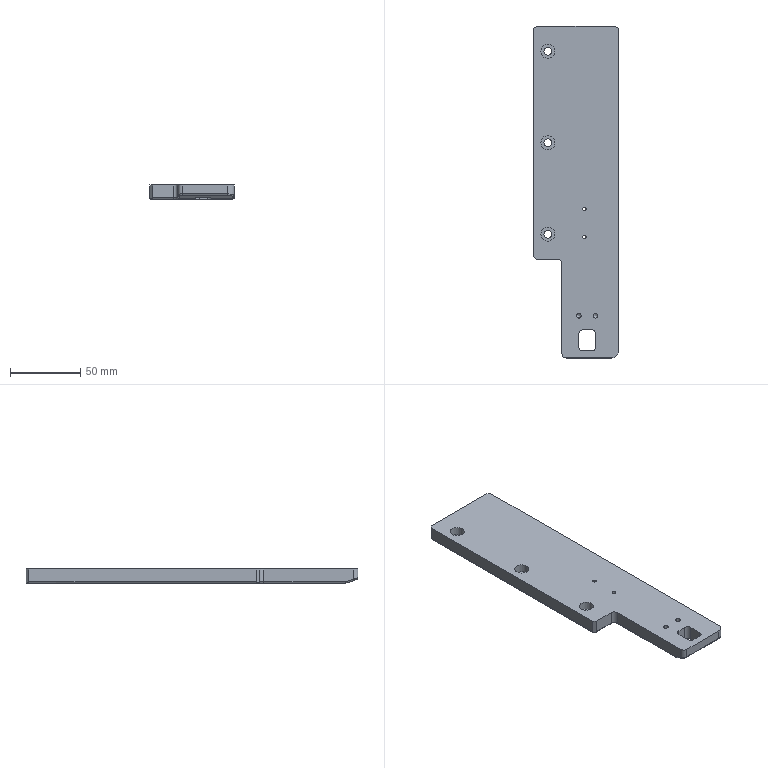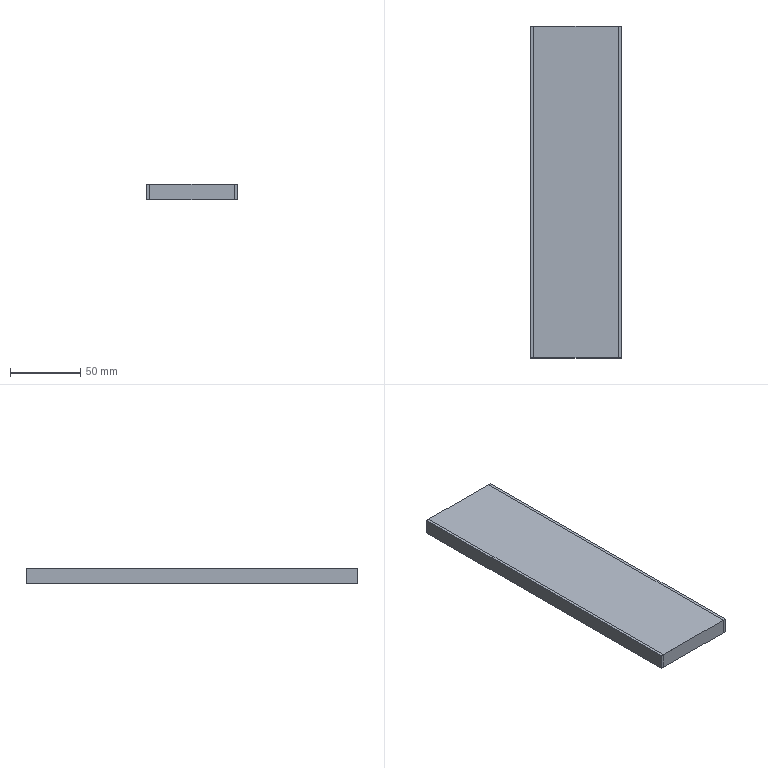CAM job | NX | 3-axis milling, drilling | part box 60 x 236 x 10 mm | stock box 64 x 236 x 11 mm
Tools:
number,name,description,diameter,corner_radius,flute_length,length,flutes
19,D80,Milling Tool-5 Parameters,80.0,0.0,50.0,75.0,2
1,D6A45,Milling Tool-5 Parameters,6.0,0.0,50.0,75.0,2
9,5.5ZT,Drilling Tool,5.5,0.0,35.0,50.0,2
2,2.5ZT,Drilling Tool,2.0,0.0,35.0,50.0,2
15,D10,Milling Tool-5 Parameters,10.0,0.0,50.0,75.0,2
14,D10JING,Milling Tool-5 Parameters,10.0,0.0,50.0,75.0,2
12,D6,Milling Tool-5 Parameters,6.0,0.0,50.0,75.0,2
17,D4R0.5,Milling Tool-5 Parameters,4.0,0.5,50.0,75.0,2
3,3.2ZT,Drilling Tool,3.2,0.0,35.0,50.0,2
Operations:
program,operation,operation_type,tool,method,geometry_group,spindle_rpm,surface_speed,feed_per_tooth,feed_cut,feed_plunge,cut_length_mm,path_length_mm,cut_time_min,machine_time_min
1,FLOOR_WALL,VolumeBased25DMillingOperation,D80,METHOD,A,6500.0,1633.0,0.1154,1500.0,100.0,332.0,386.0,0.2213,0.2267
1,DRILLING,Operation,D6A45,METHOD,A,9500.0,179.0,0.0132,250.0,0.0,24.0,285.338,0.096,0.1221
1,DRILLING_COPY_COPY,Operation,5.5ZT,METHOD,A,2000.0,21.0,0.0375,150.0,0.0,45.457,287.053,0.303,0.3272
1,DRILLING_COPY_COPY_COPY,Operation,2.5ZT,METHOD,A,2000.0,12.0,0.025,100.0,0.0,28.202,139.627,0.282,0.2932
1,ZLEVEL_PROFILE,ZLevelMilling,D10,METHOD,A,9500.0,298.0,0.1579,3000.0,1000.0,1640.781,1967.475,0.6002,0.6329
1,ZLEVEL_PROFILE_COPY,ZLevelMilling,D10,METHOD,A,9500.0,298.0,0.1579,3000.0,1000.0,1044.314,2475.02,0.4287,0.5718
1,FLOOR_WALL_1,VolumeBased25DMillingOperation,D10JING,METHOD,A,9500.0,298.0,0.0658,1250.0,100.0,231.401,614.913,0.1851,0.2235
1,ZLEVEL_PROFILE_COPY_1,ZLevelMilling,D6,METHOD,A,9500.0,179.0,0.0947,1800.0,1000.0,165.568,273.879,0.1145,0.1253
1,ZLEVEL_PROFILE_1,ZLevelMilling,D6,METHOD,A,9500.0,179.0,0.0789,1500.0,1000.0,579.277,646.277,0.3995,0.4062
1,ZLEVEL_PROFILE_2,ZLevelMilling,D4R0.5,METHOD,A,9500.0,119.0,0.1579,3000.0,100.0,11018.62,11179.672,3.673,3.689
1,ZLEVEL_PROFILE_2_COPY,ZLevelMilling,D4R0.5,METHOD,A,9500.0,119.0,0.1579,3000.0,100.0,4803.995,4974.678,1.601,1.618
1,PLANAR_MILL_COPY,PlanarMilling,D6A45,METHOD,A,9500.0,179.0,0.0658,1250.0,100.0,62.39,522.65,0.0499,0.0959
2,FLOOR_WALL_COPY,VolumeBased25DMillingOperation,D80,METHOD,B,6500.0,1633.0,0.1154,1500.0,100.0,328.0,382.0,0.2187,0.2241
2,DRILLING_COPY,Operation,D6A45,METHOD,B,9500.0,179.0,0.0132,250.0,0.0,9.6,94.569,0.0384,0.0469
2,HOLE_MILLING,CylinderMilling,D6,METHOD,B,9500.0,179.0,0.0763,1450.0,100.0,465.421,791.921,0.321,0.3536
2,DRILLING_COPY_COPY_COPY_1,Operation,3.2ZT,METHOD,B,2000.0,21.0,0.0375,150.0,0.0,23.948,123.265,0.1597,0.1696
2,PLANAR_MILL_COPY_COPY,PlanarMilling,D6A45,METHOD,B,9500.0,179.0,0.0658,1250.0,100.0,764.759,1601.59,0.6118,0.6955